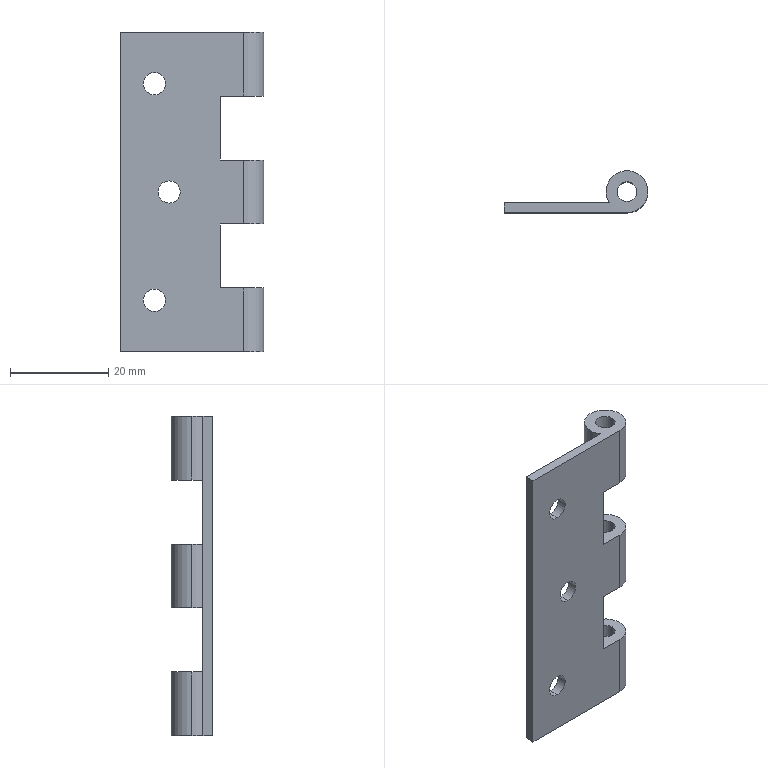Part | NX | features BREP 1 | 1 solid | 32 faces | box 29.25 x 8.5 x 65 mm | volume 4436 mm3 | cylinder 21 | plane 11 | commonest cylinder face diameters 8.5 x9 4 x6 4.5 x6
STEP:
#1=CARTESIAN_POINT('',(-18.,2.,-12.75));
#2=VERTEX_POINT('',#1);
#3=CARTESIAN_POINT('',(-18.,2.,-8.25));
#4=VERTEX_POINT('',#3);
#5=CARTESIAN_POINT('',(-18.,2.,-10.5));
#6=DIRECTION('',(0.,1.,0.));
#7=DIRECTION('',(0.,0.,1.));
#8=AXIS2_PLACEMENT_3D('',#5,#6,#7);
#9=CIRCLE('',#8,2.25);
#10=EDGE_CURVE('',#2,#4,#9,.T.);
#11=ORIENTED_EDGE('',*,*,#10,.T.);
#12=CARTESIAN_POINT('',(-18.,0.,-8.25));
#13=VERTEX_POINT('',#12);
#14=CARTESIAN_POINT('',(-18.,2.,-8.25));
#15=DIRECTION('',(0.,-1.,0.));
#16=VECTOR('',#15,1000.);
#17=LINE('',#14,#16);
#18=EDGE_CURVE('',#4,#13,#17,.T.);
#19=ORIENTED_EDGE('',*,*,#18,.T.);
#20=CARTESIAN_POINT('',(-18.,0.,-12.75));
#21=VERTEX_POINT('',#20);
#22=CARTESIAN_POINT('',(-18.,0.,-10.5));
#23=DIRECTION('',(0.,1.,0.));
#24=DIRECTION('',(0.,0.,1.));
#25=AXIS2_PLACEMENT_3D('',#22,#23,#24);
#26=CIRCLE('',#25,2.25);
#27=EDGE_CURVE('',#21,#13,#26,.T.);
#28=ORIENTED_EDGE('',*,*,#27,.F.);
#29=CARTESIAN_POINT('',(-18.,2.,-12.75));
#30=DIRECTION('',(0.,-1.,0.));
#31=VECTOR('',#30,1000.);
#32=LINE('',#29,#31);
#33=EDGE_CURVE('',#2,#21,#32,.T.);
#34=ORIENTED_EDGE('',*,*,#33,.F.);
#35=EDGE_LOOP('',(#11,#19,#28,#34));
#36=FACE_BOUND('',#35,.T.);
#37=CARTESIAN_POINT('',(-18.,2.,-10.5));
#38=DIRECTION('',(0.,-1.,0.));
#39=DIRECTION('',(0.,0.,-1.));
#40=AXIS2_PLACEMENT_3D('',#37,#38,#39);
#41=CYLINDRICAL_SURFACE('',#40,2.25);
#42=ADVANCED_FACE('',(#36),#41,.F.);
#43=CARTESIAN_POINT('',(-15.,2.,-34.75));
#44=VERTEX_POINT('',#43);
#45=CARTESIAN_POINT('',(-15.,2.,-30.25));
#46=VERTEX_POINT('',#45);
#47=CARTESIAN_POINT('',(-15.,2.,-32.5));
#48=DIRECTION('',(0.,1.,0.));
#49=DIRECTION('',(0.,0.,1.));
#50=AXIS2_PLACEMENT_3D('',#47,#48,#49);
#51=CIRCLE('',#50,2.25);
#52=EDGE_CURVE('',#44,#46,#51,.T.);
#53=ORIENTED_EDGE('',*,*,#52,.T.);
#54=CARTESIAN_POINT('',(-15.,0.,-30.25));
#55=VERTEX_POINT('',#54);
#56=CARTESIAN_POINT('',(-15.,2.,-30.25));
#57=DIRECTION('',(0.,-1.,0.));
#58=VECTOR('',#57,1000.);
#59=LINE('',#56,#58);
#60=EDGE_CURVE('',#46,#55,#59,.T.);
#61=ORIENTED_EDGE('',*,*,#60,.T.);
#62=CARTESIAN_POINT('',(-15.,0.,-34.75));
#63=VERTEX_POINT('',#62);
#64=CARTESIAN_POINT('',(-15.,0.,-32.5));
#65=DIRECTION('',(0.,1.,0.));
#66=DIRECTION('',(0.,0.,1.));
#67=AXIS2_PLACEMENT_3D('',#64,#65,#66);
#68=CIRCLE('',#67,2.25);
#69=EDGE_CURVE('',#63,#55,#68,.T.);
#70=ORIENTED_EDGE('',*,*,#69,.F.);
#71=CARTESIAN_POINT('',(-15.,2.,-34.75));
#72=DIRECTION('',(0.,-1.,0.));
#73=VECTOR('',#72,1000.);
#74=LINE('',#71,#73);
#75=EDGE_CURVE('',#44,#63,#74,.T.);
#76=ORIENTED_EDGE('',*,*,#75,.F.);
#77=EDGE_LOOP('',(#53,#61,#70,#76));
#78=FACE_BOUND('',#77,.T.);
#79=CARTESIAN_POINT('',(-15.,2.,-32.5));
#80=DIRECTION('',(0.,-1.,0.));
#81=DIRECTION('',(0.,0.,-1.));
#82=AXIS2_PLACEMENT_3D('',#79,#80,#81);
#83=CYLINDRICAL_SURFACE('',#82,2.25);
#84=ADVANCED_FACE('',(#78),#83,.F.);
#85=CARTESIAN_POINT('',(-18.,2.,-56.75));
#86=VERTEX_POINT('',#85);
#87=CARTESIAN_POINT('',(-18.,2.,-52.25));
#88=VERTEX_POINT('',#87);
#89=CARTESIAN_POINT('',(-18.,2.,-54.5));
#90=DIRECTION('',(0.,1.,0.));
#91=DIRECTION('',(0.,0.,1.));
#92=AXIS2_PLACEMENT_3D('',#89,#90,#91);
#93=CIRCLE('',#92,2.25);
#94=EDGE_CURVE('',#86,#88,#93,.T.);
#95=ORIENTED_EDGE('',*,*,#94,.T.);
#96=CARTESIAN_POINT('',(-18.,0.,-52.25));
#97=VERTEX_POINT('',#96);
#98=CARTESIAN_POINT('',(-18.,2.,-52.25));
#99=DIRECTION('',(0.,-1.,0.));
#100=VECTOR('',#99,1000.);
#101=LINE('',#98,#100);
#102=EDGE_CURVE('',#88,#97,#101,.T.);
#103=ORIENTED_EDGE('',*,*,#102,.T.);
#104=CARTESIAN_POINT('',(-18.,0.,-56.75));
#105=VERTEX_POINT('',#104);
#106=CARTESIAN_POINT('',(-18.,0.,-54.5));
#107=DIRECTION('',(0.,1.,0.));
#108=DIRECTION('',(0.,0.,1.));
#109=AXIS2_PLACEMENT_3D('',#106,#107,#108);
#110=CIRCLE('',#109,2.25);
#111=EDGE_CURVE('',#105,#97,#110,.T.);
#112=ORIENTED_EDGE('',*,*,#111,.F.);
#113=CARTESIAN_POINT('',(-18.,2.,-56.75));
#114=DIRECTION('',(0.,-1.,0.));
#115=VECTOR('',#114,1000.);
#116=LINE('',#113,#115);
#117=EDGE_CURVE('',#86,#105,#116,.T.);
#118=ORIENTED_EDGE('',*,*,#117,.F.);
#119=EDGE_LOOP('',(#95,#103,#112,#118));
#120=FACE_BOUND('',#119,.T.);
#121=CARTESIAN_POINT('',(-18.,2.,-54.5));
#122=DIRECTION('',(0.,-1.,0.));
#123=DIRECTION('',(0.,0.,-1.));
#124=AXIS2_PLACEMENT_3D('',#121,#122,#123);
#125=CYLINDRICAL_SURFACE('',#124,2.25);
#126=ADVANCED_FACE('',(#120),#125,.F.);
#127=CARTESIAN_POINT('',(-2.,4.25,-39.));
#128=VERTEX_POINT('',#127);
#129=CARTESIAN_POINT('',(2.,4.25,-39.));
#130=VERTEX_POINT('',#129);
#131=CARTESIAN_POINT('',(0.,4.25,-39.));
#132=DIRECTION('',(0.,0.,1.));
#133=DIRECTION('',(-1.,0.,0.));
#134=AXIS2_PLACEMENT_3D('',#131,#132,#133);
#135=CIRCLE('',#134,2.);
#136=EDGE_CURVE('',#128,#130,#135,.T.);
#137=ORIENTED_EDGE('',*,*,#136,.F.);
#138=CARTESIAN_POINT('',(-2.,4.25,-26.));
#139=VERTEX_POINT('',#138);
#140=CARTESIAN_POINT('',(-2.,4.25,-65.));
#141=DIRECTION('',(0.,0.,1.));
#142=VECTOR('',#141,1000.);
#143=LINE('',#140,#142);
#144=EDGE_CURVE('',#139,#128,#143,.F.);
#145=ORIENTED_EDGE('',*,*,#144,.F.);
#146=CARTESIAN_POINT('',(2.,4.25,-26.));
#147=VERTEX_POINT('',#146);
#148=CARTESIAN_POINT('',(0.,4.25,-26.));
#149=DIRECTION('',(0.,0.,-1.));
#150=DIRECTION('',(1.,0.,0.));
#151=AXIS2_PLACEMENT_3D('',#148,#149,#150);
#152=CIRCLE('',#151,2.);
#153=EDGE_CURVE('',#147,#139,#152,.T.);
#154=ORIENTED_EDGE('',*,*,#153,.F.);
#155=CARTESIAN_POINT('',(2.,4.25,-65.));
#156=DIRECTION('',(0.,0.,1.));
#157=VECTOR('',#156,1000.);
#158=LINE('',#155,#157);
#159=EDGE_CURVE('',#147,#130,#158,.F.);
#160=ORIENTED_EDGE('',*,*,#159,.T.);
#161=EDGE_LOOP('',(#137,#145,#154,#160));
#162=FACE_BOUND('',#161,.T.);
#163=CARTESIAN_POINT('',(0.,4.25,-65.));
#164=DIRECTION('',(0.,0.,1.));
#165=DIRECTION('',(1.,0.,0.));
#166=AXIS2_PLACEMENT_3D('',#163,#164,#165);
#167=CYLINDRICAL_SURFACE('',#166,2.);
#168=ADVANCED_FACE('',(#162),#167,.F.);
#169=CARTESIAN_POINT('',(-2.,4.25,-65.));
#170=VERTEX_POINT('',#169);
#171=CARTESIAN_POINT('',(2.,4.25,-65.));
#172=VERTEX_POINT('',#171);
#173=CARTESIAN_POINT('',(0.,4.25,-65.));
#174=DIRECTION('',(0.,0.,1.));
#175=DIRECTION('',(1.,0.,0.));
#176=AXIS2_PLACEMENT_3D('',#173,#174,#175);
#177=CIRCLE('',#176,2.);
#178=EDGE_CURVE('',#170,#172,#177,.T.);
#179=ORIENTED_EDGE('',*,*,#178,.F.);
#180=CARTESIAN_POINT('',(-2.,4.25,-52.));
#181=VERTEX_POINT('',#180);
#182=CARTESIAN_POINT('',(-2.,4.25,-65.));
#183=DIRECTION('',(0.,0.,1.));
#184=VECTOR('',#183,1000.);
#185=LINE('',#182,#184);
#186=EDGE_CURVE('',#181,#170,#185,.F.);
#187=ORIENTED_EDGE('',*,*,#186,.F.);
#188=CARTESIAN_POINT('',(2.,4.25,-52.));
#189=VERTEX_POINT('',#188);
#190=CARTESIAN_POINT('',(0.,4.25,-52.));
#191=DIRECTION('',(0.,0.,-1.));
#192=DIRECTION('',(1.,0.,0.));
#193=AXIS2_PLACEMENT_3D('',#190,#191,#192);
#194=CIRCLE('',#193,2.);
#195=EDGE_CURVE('',#189,#181,#194,.T.);
#196=ORIENTED_EDGE('',*,*,#195,.F.);
#197=CARTESIAN_POINT('',(2.,4.25,-65.));
#198=DIRECTION('',(0.,0.,1.));
#199=VECTOR('',#198,1000.);
#200=LINE('',#197,#199);
#201=EDGE_CURVE('',#189,#172,#200,.F.);
#202=ORIENTED_EDGE('',*,*,#201,.T.);
#203=EDGE_LOOP('',(#179,#187,#196,#202));
#204=FACE_BOUND('',#203,.T.);
#205=CARTESIAN_POINT('',(0.,4.25,-65.));
#206=DIRECTION('',(0.,0.,1.));
#207=DIRECTION('',(1.,0.,0.));
#208=AXIS2_PLACEMENT_3D('',#205,#206,#207);
#209=CYLINDRICAL_SURFACE('',#208,2.);
#210=ADVANCED_FACE('',(#204),#209,.F.);
#211=CARTESIAN_POINT('',(-2.,4.25,-13.));
#212=VERTEX_POINT('',#211);
#213=CARTESIAN_POINT('',(2.,4.25,-13.));
#214=VERTEX_POINT('',#213);
#215=CARTESIAN_POINT('',(0.,4.25,-13.));
#216=DIRECTION('',(0.,0.,1.));
#217=DIRECTION('',(-1.,0.,0.));
#218=AXIS2_PLACEMENT_3D('',#215,#216,#217);
#219=CIRCLE('',#218,2.);
#220=EDGE_CURVE('',#212,#214,#219,.T.);
#221=ORIENTED_EDGE('',*,*,#220,.F.);
#222=CARTESIAN_POINT('',(-2.,4.25,0.));
#223=VERTEX_POINT('',#222);
#224=CARTESIAN_POINT('',(-2.,4.25,-65.));
#225=DIRECTION('',(0.,0.,1.));
#226=VECTOR('',#225,1000.);
#227=LINE('',#224,#226);
#228=EDGE_CURVE('',#223,#212,#227,.F.);
#229=ORIENTED_EDGE('',*,*,#228,.F.);
#230=CARTESIAN_POINT('',(2.,4.25,0.));
#231=VERTEX_POINT('',#230);
#232=CARTESIAN_POINT('',(0.,4.25,0.));
#233=DIRECTION('',(0.,0.,1.));
#234=DIRECTION('',(1.,0.,0.));
#235=AXIS2_PLACEMENT_3D('',#232,#233,#234);
#236=CIRCLE('',#235,2.);
#237=EDGE_CURVE('',#223,#231,#236,.T.);
#238=ORIENTED_EDGE('',*,*,#237,.T.);
#239=CARTESIAN_POINT('',(2.,4.25,-65.));
#240=DIRECTION('',(0.,0.,1.));
#241=VECTOR('',#240,1000.);
#242=LINE('',#239,#241);
#243=EDGE_CURVE('',#231,#214,#242,.F.);
#244=ORIENTED_EDGE('',*,*,#243,.T.);
#245=EDGE_LOOP('',(#221,#229,#238,#244));
#246=FACE_BOUND('',#245,.T.);
#247=CARTESIAN_POINT('',(0.,4.25,-65.));
#248=DIRECTION('',(0.,0.,1.));
#249=DIRECTION('',(1.,0.,0.));
#250=AXIS2_PLACEMENT_3D('',#247,#248,#249);
#251=CYLINDRICAL_SURFACE('',#250,2.);
#252=ADVANCED_FACE('',(#246),#251,.F.);
#253=CARTESIAN_POINT('',(4.25,4.25,-39.));
#254=VERTEX_POINT('',#253);
#255=CARTESIAN_POINT('',(-4.25,4.25,-39.));
#256=VERTEX_POINT('',#255);
#257=CARTESIAN_POINT('',(0.,4.25,-39.));
#258=DIRECTION('',(0.,0.,1.));
#259=DIRECTION('',(-1.,0.,0.));
#260=AXIS2_PLACEMENT_3D('',#257,#258,#259);
#261=CIRCLE('',#260,4.25);
#262=EDGE_CURVE('',#254,#256,#261,.T.);
#263=ORIENTED_EDGE('',*,*,#262,.T.);
#264=CARTESIAN_POINT('',(-4.25,4.25,-26.));
#265=VERTEX_POINT('',#264);
#266=CARTESIAN_POINT('',(-4.25,4.25,-65.));
#267=DIRECTION('',(0.,0.,1.));
#268=VECTOR('',#267,1000.);
#269=LINE('',#266,#268);
#270=EDGE_CURVE('',#256,#265,#269,.T.);
#271=ORIENTED_EDGE('',*,*,#270,.T.);
#272=CARTESIAN_POINT('',(4.25,4.25,-26.));
#273=VERTEX_POINT('',#272);
#274=CARTESIAN_POINT('',(0.,4.25,-26.));
#275=DIRECTION('',(0.,0.,-1.));
#276=DIRECTION('',(1.,0.,0.));
#277=AXIS2_PLACEMENT_3D('',#274,#275,#276);
#278=CIRCLE('',#277,4.25);
#279=EDGE_CURVE('',#265,#273,#278,.T.);
#280=ORIENTED_EDGE('',*,*,#279,.T.);
#281=CARTESIAN_POINT('',(4.25,4.25,-65.));
#282=DIRECTION('',(0.,0.,1.));
#283=VECTOR('',#282,1000.);
#284=LINE('',#281,#283);
#285=EDGE_CURVE('',#254,#273,#284,.T.);
#286=ORIENTED_EDGE('',*,*,#285,.F.);
#287=EDGE_LOOP('',(#263,#271,#280,#286));
#288=FACE_BOUND('',#287,.T.);
#289=CARTESIAN_POINT('',(0.,4.25,-65.));
#290=DIRECTION('',(0.,0.,1.));
#291=DIRECTION('',(1.,0.,0.));
#292=AXIS2_PLACEMENT_3D('',#289,#290,#291);
#293=CYLINDRICAL_SURFACE('',#292,4.25);
#294=ADVANCED_FACE('',(#288),#293,.T.);
#295=CARTESIAN_POINT('',(0.,0.,-39.));
#296=VERTEX_POINT('',#295);
#297=CARTESIAN_POINT('',(0.,4.25,-39.));
#298=DIRECTION('',(0.,0.,1.));
#299=DIRECTION('',(-1.,0.,0.));
#300=AXIS2_PLACEMENT_3D('',#297,#298,#299);
#301=CIRCLE('',#300,4.25);
#302=EDGE_CURVE('',#296,#254,#301,.T.);
#303=ORIENTED_EDGE('',*,*,#302,.T.);
#304=ORIENTED_EDGE('',*,*,#285,.T.);
#305=CARTESIAN_POINT('',(0.,0.,-26.));
#306=VERTEX_POINT('',#305);
#307=CARTESIAN_POINT('',(0.,4.25,-26.));
#308=DIRECTION('',(0.,0.,-1.));
#309=DIRECTION('',(1.,0.,0.));
#310=AXIS2_PLACEMENT_3D('',#307,#308,#309);
#311=CIRCLE('',#310,4.25);
#312=EDGE_CURVE('',#273,#306,#311,.T.);
#313=ORIENTED_EDGE('',*,*,#312,.T.);
#314=CARTESIAN_POINT('',(0.,0.,-65.));
#315=DIRECTION('',(0.,0.,1.));
#316=VECTOR('',#315,1000.);
#317=LINE('',#314,#316);
#318=EDGE_CURVE('',#296,#306,#317,.T.);
#319=ORIENTED_EDGE('',*,*,#318,.F.);
#320=EDGE_LOOP('',(#303,#304,#313,#319));
#321=FACE_BOUND('',#320,.T.);
#322=CARTESIAN_POINT('',(0.,4.25,-65.));
#323=DIRECTION('',(0.,0.,1.));
#324=DIRECTION('',(1.,0.,0.));
#325=AXIS2_PLACEMENT_3D('',#322,#323,#324);
#326=CYLINDRICAL_SURFACE('',#325,4.25);
#327=ADVANCED_FACE('',(#321),#326,.T.);
#328=CARTESIAN_POINT('',(4.25,4.25,-65.));
#329=VERTEX_POINT('',#328);
#330=CARTESIAN_POINT('',(-4.25,4.25,-65.));
#331=VERTEX_POINT('',#330);
#332=CARTESIAN_POINT('',(0.,4.25,-65.));
#333=DIRECTION('',(0.,0.,1.));
#334=DIRECTION('',(1.,0.,0.));
#335=AXIS2_PLACEMENT_3D('',#332,#333,#334);
#336=CIRCLE('',#335,4.25);
#337=EDGE_CURVE('',#329,#331,#336,.T.);
#338=ORIENTED_EDGE('',*,*,#337,.T.);
#339=CARTESIAN_POINT('',(-4.25,4.25,-52.));
#340=VERTEX_POINT('',#339);
#341=CARTESIAN_POINT('',(-4.25,4.25,-65.));
#342=DIRECTION('',(0.,0.,1.));
#343=VECTOR('',#342,1000.);
#344=LINE('',#341,#343);
#345=EDGE_CURVE('',#331,#340,#344,.T.);
#346=ORIENTED_EDGE('',*,*,#345,.T.);
#347=CARTESIAN_POINT('',(4.25,4.25,-52.));
#348=VERTEX_POINT('',#347);
#349=CARTESIAN_POINT('',(0.,4.25,-52.));
#350=DIRECTION('',(0.,0.,-1.));
#351=DIRECTION('',(1.,0.,0.));
#352=AXIS2_PLACEMENT_3D('',#349,#350,#351);
#353=CIRCLE('',#352,4.25);
#354=EDGE_CURVE('',#340,#348,#353,.T.);
#355=ORIENTED_EDGE('',*,*,#354,.T.);
#356=CARTESIAN_POINT('',(4.25,4.25,-65.));
#357=DIRECTION('',(0.,0.,1.));
#358=VECTOR('',#357,1000.);
#359=LINE('',#356,#358);
#360=EDGE_CURVE('',#329,#348,#359,.T.);
#361=ORIENTED_EDGE('',*,*,#360,.F.);
#362=EDGE_LOOP('',(#338,#346,#355,#361));
#363=FACE_BOUND('',#362,.T.);
#364=CARTESIAN_POINT('',(0.,4.25,-65.));
#365=DIRECTION('',(0.,0.,1.));
#366=DIRECTION('',(1.,0.,0.));
#367=AXIS2_PLACEMENT_3D('',#364,#365,#366);
#368=CYLINDRICAL_SURFACE('',#367,4.25);
#369=ADVANCED_FACE('',(#363),#368,.T.);
#370=CARTESIAN_POINT('',(0.,0.,-65.));
#371=VERTEX_POINT('',#370);
#372=CARTESIAN_POINT('',(0.,4.25,-65.));
#373=DIRECTION('',(0.,0.,1.));
#374=DIRECTION('',(1.,0.,0.));
#375=AXIS2_PLACEMENT_3D('',#372,#373,#374);
#376=CIRCLE('',#375,4.25);
#377=EDGE_CURVE('',#371,#329,#376,.T.);
#378=ORIENTED_EDGE('',*,*,#377,.T.);
#379=ORIENTED_EDGE('',*,*,#360,.T.);
#380=CARTESIAN_POINT('',(0.,0.,-52.));
#381=VERTEX_POINT('',#380);
#382=CARTESIAN_POINT('',(0.,4.25,-52.));
#383=DIRECTION('',(0.,0.,-1.));
#384=DIRECTION('',(1.,0.,0.));
#385=AXIS2_PLACEMENT_3D('',#382,#383,#384);
#386=CIRCLE('',#385,4.25);
#387=EDGE_CURVE('',#348,#381,#386,.T.);
#388=ORIENTED_EDGE('',*,*,#387,.T.);
#389=CARTESIAN_POINT('',(0.,0.,-65.));
#390=DIRECTION('',(0.,0.,1.));
#391=VECTOR('',#390,1000.);
#392=LINE('',#389,#391);
#393=EDGE_CURVE('',#371,#381,#392,.T.);
#394=ORIENTED_EDGE('',*,*,#393,.F.);
#395=EDGE_LOOP('',(#378,#379,#388,#394));
#396=FACE_BOUND('',#395,.T.);
#397=CARTESIAN_POINT('',(0.,4.25,-65.));
#398=DIRECTION('',(0.,0.,1.));
#399=DIRECTION('',(1.,0.,0.));
#400=AXIS2_PLACEMENT_3D('',#397,#398,#399);
#401=CYLINDRICAL_SURFACE('',#400,4.25);
#402=ADVANCED_FACE('',(#396),#401,.T.);
#403=CARTESIAN_POINT('',(4.25,4.25,-13.));
#404=VERTEX_POINT('',#403);
#405=CARTESIAN_POINT('',(-4.25,4.25,-13.));
#406=VERTEX_POINT('',#405);
#407=CARTESIAN_POINT('',(0.,4.25,-13.));
#408=DIRECTION('',(0.,0.,1.));
#409=DIRECTION('',(-1.,0.,0.));
#410=AXIS2_PLACEMENT_3D('',#407,#408,#409);
#411=CIRCLE('',#410,4.25);
#412=EDGE_CURVE('',#404,#406,#411,.T.);
#413=ORIENTED_EDGE('',*,*,#412,.T.);
#414=CARTESIAN_POINT('',(-4.25,4.25,0.));
#415=VERTEX_POINT('',#414);
#416=CARTESIAN_POINT('',(-4.25,4.25,-65.));
#417=DIRECTION('',(0.,0.,1.));
#418=VECTOR('',#417,1000.);
#419=LINE('',#416,#418);
#420=EDGE_CURVE('',#406,#415,#419,.T.);
#421=ORIENTED_EDGE('',*,*,#420,.T.);
#422=CARTESIAN_POINT('',(4.25,4.25,0.));
#423=VERTEX_POINT('',#422);
#424=CARTESIAN_POINT('',(0.,4.25,0.));
#425=DIRECTION('',(0.,0.,1.));
#426=DIRECTION('',(1.,0.,0.));
#427=AXIS2_PLACEMENT_3D('',#424,#425,#426);
#428=CIRCLE('',#427,4.25);
#429=EDGE_CURVE('',#423,#415,#428,.T.);
#430=ORIENTED_EDGE('',*,*,#429,.F.);
#431=CARTESIAN_POINT('',(4.25,4.25,-65.));
#432=DIRECTION('',(0.,0.,1.));
#433=VECTOR('',#432,1000.);
#434=LINE('',#431,#433);
#435=EDGE_CURVE('',#404,#423,#434,.T.);
#436=ORIENTED_EDGE('',*,*,#435,.F.);
#437=EDGE_LOOP('',(#413,#421,#430,#436));
#438=FACE_BOUND('',#437,.T.);
#439=CARTESIAN_POINT('',(0.,4.25,-65.));
#440=DIRECTION('',(0.,0.,1.));
#441=DIRECTION('',(1.,0.,0.));
#442=AXIS2_PLACEMENT_3D('',#439,#440,#441);
#443=CYLINDRICAL_SURFACE('',#442,4.25);
#444=ADVANCED_FACE('',(#438),#443,.T.);
#445=CARTESIAN_POINT('',(0.,0.,-13.));
#446=VERTEX_POINT('',#445);
#447=CARTESIAN_POINT('',(0.,4.25,-13.));
#448=DIRECTION('',(0.,0.,1.));
#449=DIRECTION('',(-1.,0.,0.));
#450=AXIS2_PLACEMENT_3D('',#447,#448,#449);
#451=CIRCLE('',#450,4.25);
#452=EDGE_CURVE('',#446,#404,#451,.T.);
#453=ORIENTED_EDGE('',*,*,#452,.T.);
#454=ORIENTED_EDGE('',*,*,#435,.T.);
#455=CARTESIAN_POINT('',(0.,0.,0.));
#456=VERTEX_POINT('',#455);
#457=CARTESIAN_POINT('',(0.,4.25,0.));
#458=DIRECTION('',(0.,0.,1.));
#459=DIRECTION('',(1.,0.,0.));
#460=AXIS2_PLACEMENT_3D('',#457,#458,#459);
#461=CIRCLE('',#460,4.25);
#462=EDGE_CURVE('',#456,#423,#461,.T.);
#463=ORIENTED_EDGE('',*,*,#462,.F.);
#464=CARTESIAN_POINT('',(0.,0.,-65.));
#465=DIRECTION('',(0.,0.,1.));
#466=VECTOR('',#465,1000.);
#467=LINE('',#464,#466);
#468=EDGE_CURVE('',#446,#456,#467,.T.);
#469=ORIENTED_EDGE('',*,*,#468,.F.);
#470=EDGE_LOOP('',(#453,#454,#463,#469));
#471=FACE_BOUND('',#470,.T.);
#472=CARTESIAN_POINT('',(0.,4.25,-65.));
#473=DIRECTION('',(0.,0.,1.));
#474=DIRECTION('',(1.,0.,0.));
#475=AXIS2_PLACEMENT_3D('',#472,#473,#474);
#476=CYLINDRICAL_SURFACE('',#475,4.25);
#477=ADVANCED_FACE('',(#471),#476,.T.);
#478=CARTESIAN_POINT('',(-4.675,2.,-39.));
#479=VERTEX_POINT('',#478);
#480=CARTESIAN_POINT('',(-4.675,2.,-52.));
#481=VERTEX_POINT('',#480);
#482=CARTESIAN_POINT('',(-4.675,2.,-65.));
#483=DIRECTION('',(0.,0.,-1.));
#484=VECTOR('',#483,1000.);
#485=LINE('',#482,#484);
#486=EDGE_CURVE('',#479,#481,#485,.T.);
#487=ORIENTED_EDGE('',*,*,#486,.T.);
#488=CARTESIAN_POINT('',(-3.606,2.,-52.));
#489=VERTEX_POINT('',#488);
#490=CARTESIAN_POINT('',(-3.606,2.,-52.));
#491=DIRECTION('',(1.,0.,0.));
#492=VECTOR('',#491,1000.);
#493=LINE('',#490,#492);
#494=EDGE_CURVE('',#481,#489,#493,.T.);
#495=ORIENTED_EDGE('',*,*,#494,.T.);
#496=CARTESIAN_POINT('',(-3.606,2.,-65.));
#497=VERTEX_POINT('',#496);
#498=CARTESIAN_POINT('',(-3.606,2.,-65.));
#499=DIRECTION('',(0.,0.,1.));
#500=VECTOR('',#499,1000.);
#501=LINE('',#498,#500);
#502=EDGE_CURVE('',#497,#489,#501,.T.);
#503=ORIENTED_EDGE('',*,*,#502,.F.);
#504=CARTESIAN_POINT('',(-25.,2.,-65.));
#505=VERTEX_POINT('',#504);
#506=CARTESIAN_POINT('',(-3.606,2.,-65.));
#507=DIRECTION('',(-1.,0.,0.));
#508=VECTOR('',#507,1000.);
#509=LINE('',#506,#508);
#510=EDGE_CURVE('',#497,#505,#509,.T.);
#511=ORIENTED_EDGE('',*,*,#510,.T.);
#512=CARTESIAN_POINT('',(-25.,2.,0.));
#513=VERTEX_POINT('',#512);
#514=CARTESIAN_POINT('',(-25.,2.,-65.));
#515=DIRECTION('',(0.,0.,1.));
#516=VECTOR('',#515,1000.);
#517=LINE('',#514,#516);
#518=EDGE_CURVE('',#505,#513,#517,.T.);
#519=ORIENTED_EDGE('',*,*,#518,.T.);
#520=CARTESIAN_POINT('',(-3.606,2.,0.));
#521=VERTEX_POINT('',#520);
#522=CARTESIAN_POINT('',(-3.606,2.,0.));
#523=DIRECTION('',(-1.,0.,0.));
#524=VECTOR('',#523,1000.);
#525=LINE('',#522,#524);
#526=EDGE_CURVE('',#521,#513,#525,.T.);
#527=ORIENTED_EDGE('',*,*,#526,.F.);
#528=CARTESIAN_POINT('',(-3.606,2.,-13.));
#529=VERTEX_POINT('',#528);
#530=CARTESIAN_POINT('',(-3.606,2.,-65.));
#531=DIRECTION('',(0.,0.,1.));
#532=VECTOR('',#531,1000.);
#533=LINE('',#530,#532);
#534=EDGE_CURVE('',#529,#521,#533,.T.);
#535=ORIENTED_EDGE('',*,*,#534,.F.);
#536=CARTESIAN_POINT('',(-4.675,2.,-13.));
#537=VERTEX_POINT('',#536);
#538=CARTESIAN_POINT('',(-3.606,2.,-13.));
#539=DIRECTION('',(-1.,0.,0.));
#540=VECTOR('',#539,1000.);
#541=LINE('',#538,#540);
#542=EDGE_CURVE('',#529,#537,#541,.T.);
#543=ORIENTED_EDGE('',*,*,#542,.T.);
#544=CARTESIAN_POINT('',(-4.675,2.,-26.));
#545=VERTEX_POINT('',#544);
#546=CARTESIAN_POINT('',(-4.675,2.,-65.));
#547=DIRECTION('',(0.,0.,-1.));
#548=VECTOR('',#547,1000.);
#549=LINE('',#546,#548);
#550=EDGE_CURVE('',#537,#545,#549,.T.);
#551=ORIENTED_EDGE('',*,*,#550,.T.);
#552=CARTESIAN_POINT('',(-3.606,2.,-26.));
#553=VERTEX_POINT('',#552);
#554=CARTESIAN_POINT('',(-3.606,2.,-26.));
#555=DIRECTION('',(1.,0.,0.));
#556=VECTOR('',#555,1000.);
#557=LINE('',#554,#556);
#558=EDGE_CURVE('',#545,#553,#557,.T.);
#559=ORIENTED_EDGE('',*,*,#558,.T.);
#560=CARTESIAN_POINT('',(-3.606,2.,-39.));
#561=VERTEX_POINT('',#560);
#562=CARTESIAN_POINT('',(-3.606,2.,-65.));
#563=DIRECTION('',(0.,0.,1.));
#564=VECTOR('',#563,1000.);
#565=LINE('',#562,#564);
#566=EDGE_CURVE('',#561,#553,#565,.T.);
#567=ORIENTED_EDGE('',*,*,#566,.F.);
#568=CARTESIAN_POINT('',(-3.606,2.,-39.));
#569=DIRECTION('',(-1.,0.,0.));
#570=VECTOR('',#569,1000.);
#571=LINE('',#568,#570);
#572=EDGE_CURVE('',#561,#479,#571,.T.);
#573=ORIENTED_EDGE('',*,*,#572,.T.);
#574=EDGE_LOOP('',(#487,#495,#503,#511,#519,#527,#535,#543,#551,#559,#567,#573));
#575=FACE_BOUND('',#574,.T.);
#576=ORIENTED_EDGE('',*,*,#52,.F.);
#577=CARTESIAN_POINT('',(-15.,2.,-32.5));
#578=DIRECTION('',(0.,1.,0.));
#579=DIRECTION('',(0.,0.,1.));
#580=AXIS2_PLACEMENT_3D('',#577,#578,#579);
#581=CIRCLE('',#580,2.25);
#582=EDGE_CURVE('',#46,#44,#581,.T.);
#583=ORIENTED_EDGE('',*,*,#582,.F.);
#584=EDGE_LOOP('',(#576,#583));
#585=FACE_BOUND('',#584,.T.);
#586=ORIENTED_EDGE('',*,*,#94,.F.);
#587=CARTESIAN_POINT('',(-18.,2.,-54.5));
#588=DIRECTION('',(0.,1.,0.));
#589=DIRECTION('',(0.,0.,1.));
#590=AXIS2_PLACEMENT_3D('',#587,#588,#589);
#591=CIRCLE('',#590,2.25);
#592=EDGE_CURVE('',#88,#86,#591,.T.);
#593=ORIENTED_EDGE('',*,*,#592,.F.);
#594=EDGE_LOOP('',(#586,#593));
#595=FACE_BOUND('',#594,.T.);
#596=ORIENTED_EDGE('',*,*,#10,.F.);
#597=CARTESIAN_POINT('',(-18.,2.,-10.5));
#598=DIRECTION('',(0.,1.,0.));
#599=DIRECTION('',(0.,0.,1.));
#600=AXIS2_PLACEMENT_3D('',#597,#598,#599);
#601=CIRCLE('',#600,2.25);
#602=EDGE_CURVE('',#4,#2,#601,.T.);
#603=ORIENTED_EDGE('',*,*,#602,.F.);
#604=EDGE_LOOP('',(#596,#603));
#605=FACE_BOUND('',#604,.T.);
#606=CARTESIAN_POINT('',(-3.606,2.,-65.));
#607=DIRECTION('',(0.,1.,0.));
#608=DIRECTION('',(1.,0.,0.));
#609=AXIS2_PLACEMENT_3D('',#606,#607,#608);
#610=PLANE('',#609);
#611=ADVANCED_FACE('',(#575,#585,#595,#605),#610,.T.);
#612=ORIENTED_EDGE('',*,*,#393,.T.);
#613=CARTESIAN_POINT('',(-4.675,0.,-52.));
#614=VERTEX_POINT('',#613);
#615=CARTESIAN_POINT('',(4.675,0.,-52.));
#616=DIRECTION('',(-1.,0.,0.));
#617=VECTOR('',#616,1000.);
#618=LINE('',#615,#617);
#619=EDGE_CURVE('',#381,#614,#618,.T.);
#620=ORIENTED_EDGE('',*,*,#619,.T.);
#621=CARTESIAN_POINT('',(-4.675,0.,-39.));
#622=VERTEX_POINT('',#621);
#623=CARTESIAN_POINT('',(-4.675,0.,-52.));
#624=DIRECTION('',(0.,0.,1.));
#625=VECTOR('',#624,1000.);
#626=LINE('',#623,#625);
#627=EDGE_CURVE('',#614,#622,#626,.T.);
#628=ORIENTED_EDGE('',*,*,#627,.T.);
#629=CARTESIAN_POINT('',(-4.675,0.,-39.));
#630=DIRECTION('',(1.,0.,0.));
#631=VECTOR('',#630,1000.);
#632=LINE('',#629,#631);
#633=EDGE_CURVE('',#622,#296,#632,.T.);
#634=ORIENTED_EDGE('',*,*,#633,.T.);
#635=ORIENTED_EDGE('',*,*,#318,.T.);
#636=CARTESIAN_POINT('',(-4.675,0.,-26.));
#637=VERTEX_POINT('',#636);
#638=CARTESIAN_POINT('',(4.675,0.,-26.));
#639=DIRECTION('',(-1.,0.,0.));
#640=VECTOR('',#639,1000.);
#641=LINE('',#638,#640);
#642=EDGE_CURVE('',#306,#637,#641,.T.);
#643=ORIENTED_EDGE('',*,*,#642,.T.);
#644=CARTESIAN_POINT('',(-4.675,0.,-13.));
#645=VERTEX_POINT('',#644);
#646=CARTESIAN_POINT('',(-4.675,0.,-26.));
#647=DIRECTION('',(0.,0.,1.));
#648=VECTOR('',#647,1000.);
#649=LINE('',#646,#648);
#650=EDGE_CURVE('',#637,#645,#649,.T.);
#651=ORIENTED_EDGE('',*,*,#650,.T.);
#652=CARTESIAN_POINT('',(-4.675,0.,-13.));
#653=DIRECTION('',(1.,0.,0.));
#654=VECTOR('',#653,1000.);
#655=LINE('',#652,#654);
#656=EDGE_CURVE('',#645,#446,#655,.T.);
#657=ORIENTED_EDGE('',*,*,#656,.T.);
#658=ORIENTED_EDGE('',*,*,#468,.T.);
#659=CARTESIAN_POINT('',(-25.,0.,0.));
#660=VERTEX_POINT('',#659);
#661=CARTESIAN_POINT('',(-25.,0.,0.));
#662=DIRECTION('',(1.,0.,0.));
#663=VECTOR('',#662,1000.);
#664=LINE('',#661,#663);
#665=EDGE_CURVE('',#660,#456,#664,.T.);
#666=ORIENTED_EDGE('',*,*,#665,.F.);
#667=CARTESIAN_POINT('',(-25.,0.,-65.));
#668=VERTEX_POINT('',#667);
#669=CARTESIAN_POINT('',(-25.,0.,-65.));
#670=DIRECTION('',(0.,0.,1.));
#671=VECTOR('',#670,1000.);
#672=LINE('',#669,#671);
#673=EDGE_CURVE('',#668,#660,#672,.T.);
#674=ORIENTED_EDGE('',*,*,#673,.F.);
#675=CARTESIAN_POINT('',(-25.,0.,-65.));
#676=DIRECTION('',(1.,0.,0.));
#677=VECTOR('',#676,1000.);
#678=LINE('',#675,#677);
#679=EDGE_CURVE('',#668,#371,#678,.T.);
#680=ORIENTED_EDGE('',*,*,#679,.T.);
#681=EDGE_LOOP('',(#612,#620,#628,#634,#635,#643,#651,#657,#658,#666,#674,#680));
#682=FACE_BOUND('',#681,.T.);
#683=ORIENTED_EDGE('',*,*,#69,.T.);
#684=CARTESIAN_POINT('',(-15.,0.,-32.5));
#685=DIRECTION('',(0.,1.,0.));
#686=DIRECTION('',(0.,0.,1.));
#687=AXIS2_PLACEMENT_3D('',#684,#685,#686);
#688=CIRCLE('',#687,2.25);
#689=EDGE_CURVE('',#55,#63,#688,.T.);
#690=ORIENTED_EDGE('',*,*,#689,.T.);
#691=EDGE_LOOP('',(#683,#690));
#692=FACE_BOUND('',#691,.T.);
#693=ORIENTED_EDGE('',*,*,#111,.T.);
#694=CARTESIAN_POINT('',(-18.,0.,-54.5));
#695=DIRECTION('',(0.,1.,0.));
#696=DIRECTION('',(0.,0.,1.));
#697=AXIS2_PLACEMENT_3D('',#694,#695,#696);
#698=CIRCLE('',#697,2.25);
#699=EDGE_CURVE('',#97,#105,#698,.T.);
#700=ORIENTED_EDGE('',*,*,#699,.T.);
#701=EDGE_LOOP('',(#693,#700));
#702=FACE_BOUND('',#701,.T.);
#703=ORIENTED_EDGE('',*,*,#27,.T.);
#704=CARTESIAN_POINT('',(-18.,0.,-10.5));
#705=DIRECTION('',(0.,1.,0.));
#706=DIRECTION('',(0.,0.,1.));
#707=AXIS2_PLACEMENT_3D('',#704,#705,#706);
#708=CIRCLE('',#707,2.25);
#709=EDGE_CURVE('',#13,#21,#708,.T.);
#710=ORIENTED_EDGE('',*,*,#709,.T.);
#711=EDGE_LOOP('',(#703,#710));
#712=FACE_BOUND('',#711,.T.);
#713=CARTESIAN_POINT('',(-25.,0.,-65.));
#714=DIRECTION('',(0.,-1.,0.));
#715=DIRECTION('',(0.,0.,-1.));
#716=AXIS2_PLACEMENT_3D('',#713,#714,#715);
#717=PLANE('',#716);
#718=ADVANCED_FACE('',(#682,#692,#702,#712),#717,.T.);
#719=ORIENTED_EDGE('',*,*,#420,.F.);
#720=CARTESIAN_POINT('',(0.,4.25,-13.));
#721=DIRECTION('',(0.,0.,1.));
#722=DIRECTION('',(-1.,0.,0.));
#723=AXIS2_PLACEMENT_3D('',#720,#721,#722);
#724=CIRCLE('',#723,4.25);
#725=EDGE_CURVE('',#406,#529,#724,.T.);
#726=ORIENTED_EDGE('',*,*,#725,.T.);
#727=ORIENTED_EDGE('',*,*,#534,.T.);
#728=CARTESIAN_POINT('',(0.,4.25,0.));
#729=DIRECTION('',(0.,0.,1.));
#730=DIRECTION('',(1.,0.,0.));
#731=AXIS2_PLACEMENT_3D('',#728,#729,#730);
#732=CIRCLE('',#731,4.25);
#733=EDGE_CURVE('',#415,#521,#732,.T.);
#734=ORIENTED_EDGE('',*,*,#733,.F.);
#735=EDGE_LOOP('',(#719,#726,#727,#734));
#736=FACE_BOUND('',#735,.T.);
#737=CARTESIAN_POINT('',(0.,4.25,-65.));
#738=DIRECTION('',(0.,0.,1.));
#739=DIRECTION('',(1.,0.,0.));
#740=AXIS2_PLACEMENT_3D('',#737,#738,#739);
#741=CYLINDRICAL_SURFACE('',#740,4.25);
#742=ADVANCED_FACE('',(#736),#741,.T.);
#743=ORIENTED_EDGE('',*,*,#345,.F.);
#744=CARTESIAN_POINT('',(0.,4.25,-65.));
#745=DIRECTION('',(0.,0.,1.));
#746=DIRECTION('',(1.,0.,0.));
#747=AXIS2_PLACEMENT_3D('',#744,#745,#746);
#748=CIRCLE('',#747,4.25);
#749=EDGE_CURVE('',#331,#497,#748,.T.);
#750=ORIENTED_EDGE('',*,*,#749,.T.);
#751=ORIENTED_EDGE('',*,*,#502,.T.);
#752=CARTESIAN_POINT('',(0.,4.25,-52.));
#753=DIRECTION('',(0.,0.,-1.));
#754=DIRECTION('',(1.,0.,0.));
#755=AXIS2_PLACEMENT_3D('',#752,#753,#754);
#756=CIRCLE('',#755,4.25);
#757=EDGE_CURVE('',#489,#340,#756,.T.);
#758=ORIENTED_EDGE('',*,*,#757,.T.);
#759=EDGE_LOOP('',(#743,#750,#751,#758));
#760=FACE_BOUND('',#759,.T.);
#761=CARTESIAN_POINT('',(0.,4.25,-65.));
#762=DIRECTION('',(0.,0.,1.));
#763=DIRECTION('',(1.,0.,0.));
#764=AXIS2_PLACEMENT_3D('',#761,#762,#763);
#765=CYLINDRICAL_SURFACE('',#764,4.25);
#766=ADVANCED_FACE('',(#760),#765,.T.);
#767=ORIENTED_EDGE('',*,*,#270,.F.);
#768=CARTESIAN_POINT('',(0.,4.25,-39.));
#769=DIRECTION('',(0.,0.,1.));
#770=DIRECTION('',(-1.,0.,0.));
#771=AXIS2_PLACEMENT_3D('',#768,#769,#770);
#772=CIRCLE('',#771,4.25);
#773=EDGE_CURVE('',#256,#561,#772,.T.);
#774=ORIENTED_EDGE('',*,*,#773,.T.);
#775=ORIENTED_EDGE('',*,*,#566,.T.);
#776=CARTESIAN_POINT('',(0.,4.25,-26.));
#777=DIRECTION('',(0.,0.,-1.));
#778=DIRECTION('',(1.,0.,0.));
#779=AXIS2_PLACEMENT_3D('',#776,#777,#778);
#780=CIRCLE('',#779,4.25);
#781=EDGE_CURVE('',#553,#265,#780,.T.);
#782=ORIENTED_EDGE('',*,*,#781,.T.);
#783=EDGE_LOOP('',(#767,#774,#775,#782));
#784=FACE_BOUND('',#783,.T.);
#785=CARTESIAN_POINT('',(0.,4.25,-65.));
#786=DIRECTION('',(0.,0.,1.));
#787=DIRECTION('',(1.,0.,0.));
#788=AXIS2_PLACEMENT_3D('',#785,#786,#787);
#789=CYLINDRICAL_SURFACE('',#788,4.25);
#790=ADVANCED_FACE('',(#784),#789,.T.);
#791=ORIENTED_EDGE('',*,*,#228,.T.);
#792=CARTESIAN_POINT('',(0.,4.25,-13.));
#793=DIRECTION('',(0.,0.,1.));
#794=DIRECTION('',(-1.,0.,0.));
#795=AXIS2_PLACEMENT_3D('',#792,#793,#794);
#796=CIRCLE('',#795,2.);
#797=EDGE_CURVE('',#214,#212,#796,.T.);
#798=ORIENTED_EDGE('',*,*,#797,.F.);
#799=ORIENTED_EDGE('',*,*,#243,.F.);
#800=CARTESIAN_POINT('',(0.,4.25,0.));
#801=DIRECTION('',(0.,0.,1.));
#802=DIRECTION('',(1.,0.,0.));
#803=AXIS2_PLACEMENT_3D('',#800,#801,#802);
#804=CIRCLE('',#803,2.);
#805=EDGE_CURVE('',#231,#223,#804,.T.);
#806=ORIENTED_EDGE('',*,*,#805,.T.);
#807=EDGE_LOOP('',(#791,#798,#799,#806));
#808=FACE_BOUND('',#807,.T.);
#809=CARTESIAN_POINT('',(0.,4.25,-65.));
#810=DIRECTION('',(0.,0.,1.));
#811=DIRECTION('',(1.,0.,0.));
#812=AXIS2_PLACEMENT_3D('',#809,#810,#811);
#813=CYLINDRICAL_SURFACE('',#812,2.);
#814=ADVANCED_FACE('',(#808),#813,.F.);
#815=ORIENTED_EDGE('',*,*,#186,.T.);
#816=CARTESIAN_POINT('',(0.,4.25,-65.));
#817=DIRECTION('',(0.,0.,1.));
#818=DIRECTION('',(1.,0.,0.));
#819=AXIS2_PLACEMENT_3D('',#816,#817,#818);
#820=CIRCLE('',#819,2.);
#821=EDGE_CURVE('',#172,#170,#820,.T.);
#822=ORIENTED_EDGE('',*,*,#821,.F.);
#823=ORIENTED_EDGE('',*,*,#201,.F.);
#824=CARTESIAN_POINT('',(0.,4.25,-52.));
#825=DIRECTION('',(0.,0.,-1.));
#826=DIRECTION('',(1.,0.,0.));
#827=AXIS2_PLACEMENT_3D('',#824,#825,#826);
#828=CIRCLE('',#827,2.);
#829=EDGE_CURVE('',#181,#189,#828,.T.);
#830=ORIENTED_EDGE('',*,*,#829,.F.);
#831=EDGE_LOOP('',(#815,#822,#823,#830));
#832=FACE_BOUND('',#831,.T.);
#833=CARTESIAN_POINT('',(0.,4.25,-65.));
#834=DIRECTION('',(0.,0.,1.));
#835=DIRECTION('',(1.,0.,0.));
#836=AXIS2_PLACEMENT_3D('',#833,#834,#835);
#837=CYLINDRICAL_SURFACE('',#836,2.);
#838=ADVANCED_FACE('',(#832),#837,.F.);
#839=CARTESIAN_POINT('',(-25.,2.,0.));
#840=DIRECTION('',(0.,-1.,0.));
#841=VECTOR('',#840,1000.);
#842=LINE('',#839,#841);
#843=EDGE_CURVE('',#513,#660,#842,.T.);
#844=ORIENTED_EDGE('',*,*,#843,.F.);
#845=ORIENTED_EDGE('',*,*,#518,.F.);
#846=CARTESIAN_POINT('',(-25.,2.,-65.));
#847=DIRECTION('',(0.,-1.,0.));
#848=VECTOR('',#847,1000.);
#849=LINE('',#846,#848);
#850=EDGE_CURVE('',#505,#668,#849,.T.);
#851=ORIENTED_EDGE('',*,*,#850,.T.);
#852=ORIENTED_EDGE('',*,*,#673,.T.);
#853=EDGE_LOOP('',(#844,#845,#851,#852));
#854=FACE_BOUND('',#853,.T.);
#855=CARTESIAN_POINT('',(-25.,2.,-65.));
#856=DIRECTION('',(-1.,0.,0.));
#857=DIRECTION('',(0.,0.,1.));
#858=AXIS2_PLACEMENT_3D('',#855,#856,#857);
#859=PLANE('',#858);
#860=ADVANCED_FACE('',(#854),#859,.T.);
#861=ORIENTED_EDGE('',*,*,#850,.F.);
#862=ORIENTED_EDGE('',*,*,#510,.F.);
#863=ORIENTED_EDGE('',*,*,#749,.F.);
#864=ORIENTED_EDGE('',*,*,#337,.F.);
#865=ORIENTED_EDGE('',*,*,#377,.F.);
#866=ORIENTED_EDGE('',*,*,#679,.F.);
#867=EDGE_LOOP('',(#861,#862,#863,#864,#865,#866));
#868=FACE_BOUND('',#867,.T.);
#869=ORIENTED_EDGE('',*,*,#821,.T.);
#870=ORIENTED_EDGE('',*,*,#178,.T.);
#871=EDGE_LOOP('',(#869,#870));
#872=FACE_BOUND('',#871,.T.);
#873=CARTESIAN_POINT('',(0.,4.25,-65.));
#874=DIRECTION('',(0.,0.,1.));
#875=DIRECTION('',(1.,0.,0.));
#876=AXIS2_PLACEMENT_3D('',#873,#874,#875);
#877=PLANE('',#876);
#878=ADVANCED_FACE('',(#868,#872),#877,.F.);
#879=ORIENTED_EDGE('',*,*,#843,.T.);
#880=ORIENTED_EDGE('',*,*,#665,.T.);
#881=ORIENTED_EDGE('',*,*,#462,.T.);
#882=ORIENTED_EDGE('',*,*,#429,.T.);
#883=ORIENTED_EDGE('',*,*,#733,.T.);
#884=ORIENTED_EDGE('',*,*,#526,.T.);
#885=EDGE_LOOP('',(#879,#880,#881,#882,#883,#884));
#886=FACE_BOUND('',#885,.T.);
#887=ORIENTED_EDGE('',*,*,#805,.F.);
#888=ORIENTED_EDGE('',*,*,#237,.F.);
#889=EDGE_LOOP('',(#887,#888));
#890=FACE_BOUND('',#889,.T.);
#891=CARTESIAN_POINT('',(0.,4.25,0.));
#892=DIRECTION('',(0.,0.,1.));
#893=DIRECTION('',(1.,0.,0.));
#894=AXIS2_PLACEMENT_3D('',#891,#892,#893);
#895=PLANE('',#894);
#896=ADVANCED_FACE('',(#886,#890),#895,.T.);
#897=CARTESIAN_POINT('',(-4.675,8.5,-26.));
#898=DIRECTION('',(0.,-1.,0.));
#899=VECTOR('',#898,1000.);
#900=LINE('',#897,#899);
#901=EDGE_CURVE('',#545,#637,#900,.T.);
#902=ORIENTED_EDGE('',*,*,#901,.T.);
#903=ORIENTED_EDGE('',*,*,#642,.F.);
#904=ORIENTED_EDGE('',*,*,#312,.F.);
#905=ORIENTED_EDGE('',*,*,#279,.F.);
#906=ORIENTED_EDGE('',*,*,#781,.F.);
#907=ORIENTED_EDGE('',*,*,#558,.F.);
#908=EDGE_LOOP('',(#902,#903,#904,#905,#906,#907));
#909=FACE_BOUND('',#908,.T.);
#910=ORIENTED_EDGE('',*,*,#153,.T.);
#911=CARTESIAN_POINT('',(0.,4.25,-26.));
#912=DIRECTION('',(0.,0.,-1.));
#913=DIRECTION('',(1.,0.,0.));
#914=AXIS2_PLACEMENT_3D('',#911,#912,#913);
#915=CIRCLE('',#914,2.);
#916=EDGE_CURVE('',#139,#147,#915,.T.);
#917=ORIENTED_EDGE('',*,*,#916,.T.);
#918=EDGE_LOOP('',(#910,#917));
#919=FACE_BOUND('',#918,.T.);
#920=CARTESIAN_POINT('',(4.675,8.5,-26.));
#921=DIRECTION('',(0.,0.,1.));
#922=DIRECTION('',(1.,0.,0.));
#923=AXIS2_PLACEMENT_3D('',#920,#921,#922);
#924=PLANE('',#923);
#925=ADVANCED_FACE('',(#909,#919),#924,.T.);
#926=ORIENTED_EDGE('',*,*,#452,.F.);
#927=ORIENTED_EDGE('',*,*,#656,.F.);
#928=CARTESIAN_POINT('',(-4.675,8.5,-13.));
#929=DIRECTION('',(0.,-1.,0.));
#930=VECTOR('',#929,1000.);
#931=LINE('',#928,#930);
#932=EDGE_CURVE('',#537,#645,#931,.T.);
#933=ORIENTED_EDGE('',*,*,#932,.F.);
#934=ORIENTED_EDGE('',*,*,#542,.F.);
#935=ORIENTED_EDGE('',*,*,#725,.F.);
#936=ORIENTED_EDGE('',*,*,#412,.F.);
#937=EDGE_LOOP('',(#926,#927,#933,#934,#935,#936));
#938=FACE_BOUND('',#937,.T.);
#939=ORIENTED_EDGE('',*,*,#797,.T.);
#940=ORIENTED_EDGE('',*,*,#220,.T.);
#941=EDGE_LOOP('',(#939,#940));
#942=FACE_BOUND('',#941,.T.);
#943=CARTESIAN_POINT('',(-4.675,8.5,-13.));
#944=DIRECTION('',(0.,0.,-1.));
#945=DIRECTION('',(0.,-1.,0.));
#946=AXIS2_PLACEMENT_3D('',#943,#944,#945);
#947=PLANE('',#946);
#948=ADVANCED_FACE('',(#938,#942),#947,.T.);
#949=ORIENTED_EDGE('',*,*,#932,.T.);
#950=ORIENTED_EDGE('',*,*,#650,.F.);
#951=ORIENTED_EDGE('',*,*,#901,.F.);
#952=ORIENTED_EDGE('',*,*,#550,.F.);
#953=EDGE_LOOP('',(#949,#950,#951,#952));
#954=FACE_BOUND('',#953,.T.);
#955=CARTESIAN_POINT('',(-4.675,8.5,-26.));
#956=DIRECTION('',(1.,0.,0.));
#957=DIRECTION('',(0.,1.,0.));
#958=AXIS2_PLACEMENT_3D('',#955,#956,#957);
#959=PLANE('',#958);
#960=ADVANCED_FACE('',(#954),#959,.T.);
#961=CARTESIAN_POINT('',(-4.675,8.5,-52.));
#962=DIRECTION('',(0.,-1.,0.));
#963=VECTOR('',#962,1000.);
#964=LINE('',#961,#963);
#965=EDGE_CURVE('',#481,#614,#964,.T.);
#966=ORIENTED_EDGE('',*,*,#965,.T.);
#967=ORIENTED_EDGE('',*,*,#619,.F.);
#968=ORIENTED_EDGE('',*,*,#387,.F.);
#969=ORIENTED_EDGE('',*,*,#354,.F.);
#970=ORIENTED_EDGE('',*,*,#757,.F.);
#971=ORIENTED_EDGE('',*,*,#494,.F.);
#972=EDGE_LOOP('',(#966,#967,#968,#969,#970,#971));
#973=FACE_BOUND('',#972,.T.);
#974=ORIENTED_EDGE('',*,*,#195,.T.);
#975=ORIENTED_EDGE('',*,*,#829,.T.);
#976=EDGE_LOOP('',(#974,#975));
#977=FACE_BOUND('',#976,.T.);
#978=CARTESIAN_POINT('',(4.675,8.5,-52.));
#979=DIRECTION('',(0.,0.,1.));
#980=DIRECTION('',(1.,0.,0.));
#981=AXIS2_PLACEMENT_3D('',#978,#979,#980);
#982=PLANE('',#981);
#983=ADVANCED_FACE('',(#973,#977),#982,.T.);
#984=ORIENTED_EDGE('',*,*,#302,.F.);
#985=ORIENTED_EDGE('',*,*,#633,.F.);
#986=CARTESIAN_POINT('',(-4.675,8.5,-39.));
#987=DIRECTION('',(0.,-1.,0.));
#988=VECTOR('',#987,1000.);
#989=LINE('',#986,#988);
#990=EDGE_CURVE('',#479,#622,#989,.T.);
#991=ORIENTED_EDGE('',*,*,#990,.F.);
#992=ORIENTED_EDGE('',*,*,#572,.F.);
#993=ORIENTED_EDGE('',*,*,#773,.F.);
#994=ORIENTED_EDGE('',*,*,#262,.F.);
#995=EDGE_LOOP('',(#984,#985,#991,#992,#993,#994));
#996=FACE_BOUND('',#995,.T.);
#997=CARTESIAN_POINT('',(0.,4.25,-39.));
#998=DIRECTION('',(0.,0.,1.));
#999=DIRECTION('',(-1.,0.,0.));
#1000=AXIS2_PLACEMENT_3D('',#997,#998,#999);
#1001=CIRCLE('',#1000,2.);
#1002=EDGE_CURVE('',#130,#128,#1001,.T.);
#1003=ORIENTED_EDGE('',*,*,#1002,.T.);
#1004=ORIENTED_EDGE('',*,*,#136,.T.);
#1005=EDGE_LOOP('',(#1003,#1004));
#1006=FACE_BOUND('',#1005,.T.);
#1007=CARTESIAN_POINT('',(-4.675,8.5,-39.));
#1008=DIRECTION('',(0.,0.,-1.));
#1009=DIRECTION('',(0.,-1.,0.));
#1010=AXIS2_PLACEMENT_3D('',#1007,#1008,#1009);
#1011=PLANE('',#1010);
#1012=ADVANCED_FACE('',(#996,#1006),#1011,.T.);
#1013=ORIENTED_EDGE('',*,*,#990,.T.);
#1014=ORIENTED_EDGE('',*,*,#627,.F.);
#1015=ORIENTED_EDGE('',*,*,#965,.F.);
#1016=ORIENTED_EDGE('',*,*,#486,.F.);
#1017=EDGE_LOOP('',(#1013,#1014,#1015,#1016));
#1018=FACE_BOUND('',#1017,.T.);
#1019=CARTESIAN_POINT('',(-4.675,8.5,-52.));
#1020=DIRECTION('',(1.,0.,0.));
#1021=DIRECTION('',(0.,1.,0.));
#1022=AXIS2_PLACEMENT_3D('',#1019,#1020,#1021);
#1023=PLANE('',#1022);
#1024=ADVANCED_FACE('',(#1018),#1023,.T.);
#1025=ORIENTED_EDGE('',*,*,#144,.T.);
#1026=ORIENTED_EDGE('',*,*,#1002,.F.);
#1027=ORIENTED_EDGE('',*,*,#159,.F.);
#1028=ORIENTED_EDGE('',*,*,#916,.F.);
#1029=EDGE_LOOP('',(#1025,#1026,#1027,#1028));
#1030=FACE_BOUND('',#1029,.T.);
#1031=CARTESIAN_POINT('',(0.,4.25,-65.));
#1032=DIRECTION('',(0.,0.,1.));
#1033=DIRECTION('',(1.,0.,0.));
#1034=AXIS2_PLACEMENT_3D('',#1031,#1032,#1033);
#1035=CYLINDRICAL_SURFACE('',#1034,2.);
#1036=ADVANCED_FACE('',(#1030),#1035,.F.);
#1037=ORIENTED_EDGE('',*,*,#102,.F.);
#1038=ORIENTED_EDGE('',*,*,#592,.T.);
#1039=ORIENTED_EDGE('',*,*,#117,.T.);
#1040=ORIENTED_EDGE('',*,*,#699,.F.);
#1041=EDGE_LOOP('',(#1037,#1038,#1039,#1040));
#1042=FACE_BOUND('',#1041,.T.);
#1043=CARTESIAN_POINT('',(-18.,2.,-54.5));
#1044=DIRECTION('',(0.,-1.,0.));
#1045=DIRECTION('',(0.,0.,-1.));
#1046=AXIS2_PLACEMENT_3D('',#1043,#1044,#1045);
#1047=CYLINDRICAL_SURFACE('',#1046,2.25);
#1048=ADVANCED_FACE('',(#1042),#1047,.F.);
#1049=ORIENTED_EDGE('',*,*,#60,.F.);
#1050=ORIENTED_EDGE('',*,*,#582,.T.);
#1051=ORIENTED_EDGE('',*,*,#75,.T.);
#1052=ORIENTED_EDGE('',*,*,#689,.F.);
#1053=EDGE_LOOP('',(#1049,#1050,#1051,#1052));
#1054=FACE_BOUND('',#1053,.T.);
#1055=CARTESIAN_POINT('',(-15.,2.,-32.5));
#1056=DIRECTION('',(0.,-1.,0.));
#1057=DIRECTION('',(0.,0.,-1.));
#1058=AXIS2_PLACEMENT_3D('',#1055,#1056,#1057);
#1059=CYLINDRICAL_SURFACE('',#1058,2.25);
#1060=ADVANCED_FACE('',(#1054),#1059,.F.);
#1061=ORIENTED_EDGE('',*,*,#18,.F.);
#1062=ORIENTED_EDGE('',*,*,#602,.T.);
#1063=ORIENTED_EDGE('',*,*,#33,.T.);
#1064=ORIENTED_EDGE('',*,*,#709,.F.);
#1065=EDGE_LOOP('',(#1061,#1062,#1063,#1064));
#1066=FACE_BOUND('',#1065,.T.);
#1067=CARTESIAN_POINT('',(-18.,2.,-10.5));
#1068=DIRECTION('',(0.,-1.,0.));
#1069=DIRECTION('',(0.,0.,-1.));
#1070=AXIS2_PLACEMENT_3D('',#1067,#1068,#1069);
#1071=CYLINDRICAL_SURFACE('',#1070,2.25);
#1072=ADVANCED_FACE('',(#1066),#1071,.F.);
#1073=CLOSED_SHELL('',(#42,#84,#126,#168,#210,#252,#294,#327,#369,#402,#444,#477,#611,#718,#742,#766,#790,#814,#838,#860,#878,#896,#925,#948,#960,#983,#1012,#1024,#1036,#1048,#1060,#1072));
#1074=MANIFOLD_SOLID_BREP('',#1073);
#1075=(LENGTH_UNIT()NAMED_UNIT(*)SI_UNIT(.MILLI.,.METRE.));
#1076=UNCERTAINTY_MEASURE_WITH_UNIT(LENGTH_MEASURE(0.00001),#1075,'','');
#1077=(NAMED_UNIT(*)PLANE_ANGLE_UNIT()SI_UNIT($,.RADIAN.));
#1078=(NAMED_UNIT(*)SI_UNIT($,.STERADIAN.)SOLID_ANGLE_UNIT());
#1079=(GEOMETRIC_REPRESENTATION_CONTEXT(3)GLOBAL_UNCERTAINTY_ASSIGNED_CONTEXT((#1076))GLOBAL_UNIT_ASSIGNED_CONTEXT((#1075,#1077,#1078))REPRESENTATION_CONTEXT('',''));
#1080=ADVANCED_BREP_SHAPE_REPRESENTATION('',(#1074),#1079);